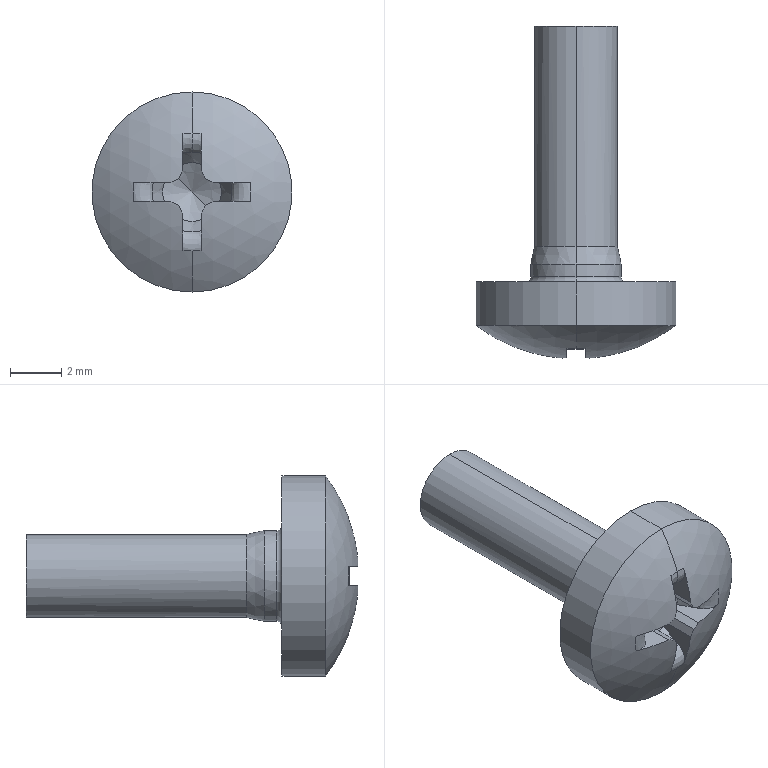Part | STEP file | 4-20.sldasm-Part-186 | 1 solid | 41 faces | box 7.82 x 12.968 x 7.82 mm | volume 191.707 mm3 | plane 18 | cone 8 | torus 7 | cylinder 6 | sphere 2 | commonest cylinder face diameters 3.241 x2 3.545 x2 7.82 x2